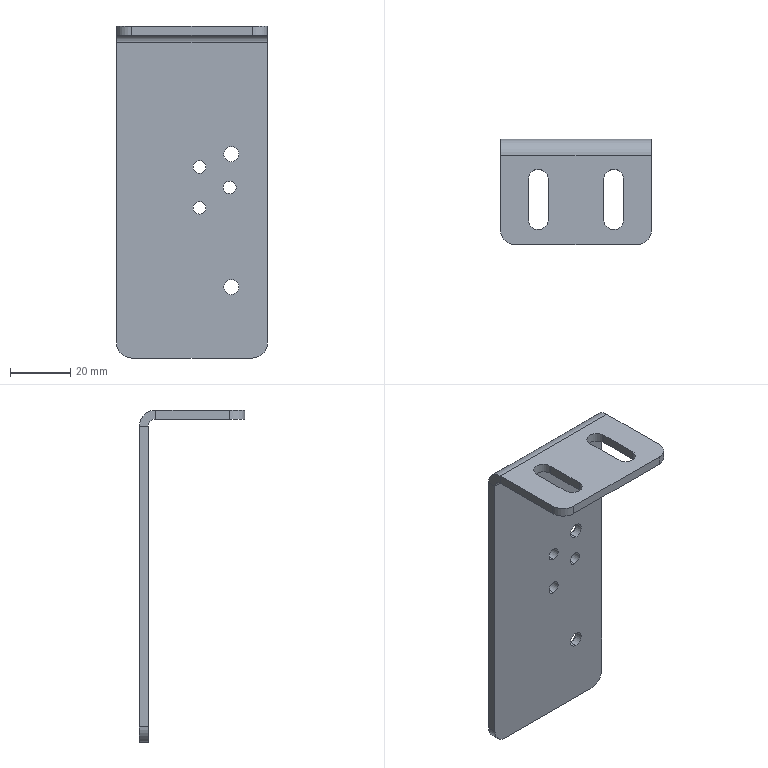Part | STEP file | 1 solid | 40 faces | box 50 x 35 x 110 mm | volume 19995 mm3 | cylinder 20 | plane 16 | cone 4 | commonest cylinder face diameters 4.2 x6 5 x5 6.6 x4 10 x4 11 x1